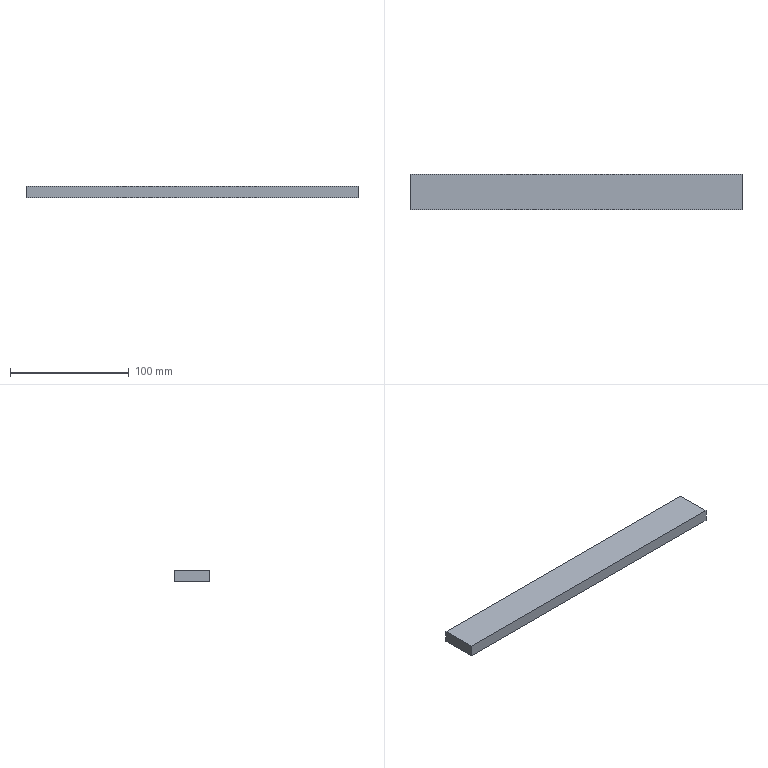Part | NX | features solid 2 | 1 solid | 6 faces | box 279 x 30 x 10 mm | volume 83700 mm3 | plane 6
STEP:
#1=CARTESIAN_POINT('',(-509.173,490.,-20.));
#2=VERTEX_POINT('',#1);
#3=CARTESIAN_POINT('',(-509.173,490.,-30.));
#4=VERTEX_POINT('',#3);
#5=CARTESIAN_POINT('',(-509.173,490.,-10.));
#6=DIRECTION('',(0.,0.,1.));
#7=VECTOR('',#6,1000.);
#8=LINE('',#5,#7);
#9=EDGE_CURVE('',#2,#4,#8,.F.);
#10=ORIENTED_EDGE('',*,*,#9,.F.);
#11=CARTESIAN_POINT('',(-230.173,490.,-20.));
#12=VERTEX_POINT('',#11);
#13=CARTESIAN_POINT('',(-295.173,490.,-20.));
#14=DIRECTION('',(-1.,0.,0.));
#15=VECTOR('',#14,1000.);
#16=LINE('',#13,#15);
#17=EDGE_CURVE('',#12,#2,#16,.T.);
#18=ORIENTED_EDGE('',*,*,#17,.F.);
#19=CARTESIAN_POINT('',(-230.173,490.,-30.));
#20=VERTEX_POINT('',#19);
#21=CARTESIAN_POINT('',(-230.173,490.,-10.));
#22=DIRECTION('',(0.,0.,1.));
#23=VECTOR('',#22,1000.);
#24=LINE('',#21,#23);
#25=EDGE_CURVE('',#12,#20,#24,.F.);
#26=ORIENTED_EDGE('',*,*,#25,.T.);
#27=CARTESIAN_POINT('',(-295.173,490.,-30.));
#28=DIRECTION('',(1.,0.,0.));
#29=VECTOR('',#28,1000.);
#30=LINE('',#27,#29);
#31=EDGE_CURVE('',#20,#4,#30,.F.);
#32=ORIENTED_EDGE('',*,*,#31,.T.);
#33=EDGE_LOOP('',(#10,#18,#26,#32));
#34=FACE_BOUND('',#33,.T.);
#35=CARTESIAN_POINT('',(-295.173,490.,-10.));
#36=DIRECTION('',(0.,-1.,0.));
#37=DIRECTION('',(1.,0.,0.));
#38=AXIS2_PLACEMENT_3D('',#35,#36,#37);
#39=PLANE('',#38);
#40=ADVANCED_FACE('',(#34),#39,.F.);
#41=CARTESIAN_POINT('',(-509.173,460.,-30.));
#42=VERTEX_POINT('',#41);
#43=CARTESIAN_POINT('',(-509.173,460.,-20.));
#44=VERTEX_POINT('',#43);
#45=CARTESIAN_POINT('',(-509.173,460.,-10.));
#46=DIRECTION('',(0.,0.,1.));
#47=VECTOR('',#46,1000.);
#48=LINE('',#45,#47);
#49=EDGE_CURVE('',#42,#44,#48,.T.);
#50=ORIENTED_EDGE('',*,*,#49,.F.);
#51=CARTESIAN_POINT('',(-230.173,460.,-30.));
#52=VERTEX_POINT('',#51);
#53=CARTESIAN_POINT('',(-374.173,460.,-30.));
#54=DIRECTION('',(1.,0.,0.));
#55=VECTOR('',#54,1000.);
#56=LINE('',#53,#55);
#57=EDGE_CURVE('',#42,#52,#56,.T.);
#58=ORIENTED_EDGE('',*,*,#57,.T.);
#59=CARTESIAN_POINT('',(-230.173,460.,-20.));
#60=VERTEX_POINT('',#59);
#61=CARTESIAN_POINT('',(-230.173,460.,-10.));
#62=DIRECTION('',(0.,0.,1.));
#63=VECTOR('',#62,1000.);
#64=LINE('',#61,#63);
#65=EDGE_CURVE('',#52,#60,#64,.T.);
#66=ORIENTED_EDGE('',*,*,#65,.T.);
#67=CARTESIAN_POINT('',(-295.173,460.,-20.));
#68=DIRECTION('',(-1.,0.,0.));
#69=VECTOR('',#68,1000.);
#70=LINE('',#67,#69);
#71=EDGE_CURVE('',#60,#44,#70,.T.);
#72=ORIENTED_EDGE('',*,*,#71,.T.);
#73=EDGE_LOOP('',(#50,#58,#66,#72));
#74=FACE_BOUND('',#73,.T.);
#75=CARTESIAN_POINT('',(-295.173,460.,-10.));
#76=DIRECTION('',(0.,-1.,0.));
#77=DIRECTION('',(1.,0.,0.));
#78=AXIS2_PLACEMENT_3D('',#75,#76,#77);
#79=PLANE('',#78);
#80=ADVANCED_FACE('',(#74),#79,.T.);
#81=ORIENTED_EDGE('',*,*,#65,.F.);
#82=CARTESIAN_POINT('',(-230.173,490.,-30.));
#83=DIRECTION('',(0.,1.,0.));
#84=VECTOR('',#83,1000.);
#85=LINE('',#82,#84);
#86=EDGE_CURVE('',#20,#52,#85,.F.);
#87=ORIENTED_EDGE('',*,*,#86,.F.);
#88=ORIENTED_EDGE('',*,*,#25,.F.);
#89=CARTESIAN_POINT('',(-230.173,460.,-20.));
#90=DIRECTION('',(0.,-1.,0.));
#91=VECTOR('',#90,1000.);
#92=LINE('',#89,#91);
#93=EDGE_CURVE('',#12,#60,#92,.T.);
#94=ORIENTED_EDGE('',*,*,#93,.T.);
#95=EDGE_LOOP('',(#81,#87,#88,#94));
#96=FACE_BOUND('',#95,.T.);
#97=CARTESIAN_POINT('',(-230.173,490.,-10.));
#98=DIRECTION('',(-1.,0.,0.));
#99=DIRECTION('',(0.,0.,1.));
#100=AXIS2_PLACEMENT_3D('',#97,#98,#99);
#101=PLANE('',#100);
#102=ADVANCED_FACE('',(#96),#101,.F.);
#103=CARTESIAN_POINT('',(-509.173,490.,-30.));
#104=DIRECTION('',(0.,1.,0.));
#105=VECTOR('',#104,1000.);
#106=LINE('',#103,#105);
#107=EDGE_CURVE('',#4,#42,#106,.F.);
#108=ORIENTED_EDGE('',*,*,#107,.T.);
#109=ORIENTED_EDGE('',*,*,#49,.T.);
#110=CARTESIAN_POINT('',(-509.173,460.,-20.));
#111=DIRECTION('',(0.,-1.,0.));
#112=VECTOR('',#111,1000.);
#113=LINE('',#110,#112);
#114=EDGE_CURVE('',#2,#44,#113,.T.);
#115=ORIENTED_EDGE('',*,*,#114,.F.);
#116=ORIENTED_EDGE('',*,*,#9,.T.);
#117=EDGE_LOOP('',(#108,#109,#115,#116));
#118=FACE_BOUND('',#117,.T.);
#119=CARTESIAN_POINT('',(-509.173,490.,-10.));
#120=DIRECTION('',(-1.,0.,0.));
#121=DIRECTION('',(0.,0.,1.));
#122=AXIS2_PLACEMENT_3D('',#119,#120,#121);
#123=PLANE('',#122);
#124=ADVANCED_FACE('',(#118),#123,.T.);
#125=ORIENTED_EDGE('',*,*,#57,.F.);
#126=ORIENTED_EDGE('',*,*,#107,.F.);
#127=ORIENTED_EDGE('',*,*,#31,.F.);
#128=ORIENTED_EDGE('',*,*,#86,.T.);
#129=EDGE_LOOP('',(#125,#126,#127,#128));
#130=FACE_BOUND('',#129,.T.);
#131=CARTESIAN_POINT('',(-374.173,460.,-30.));
#132=DIRECTION('',(0.,0.,1.));
#133=DIRECTION('',(1.,0.,0.));
#134=AXIS2_PLACEMENT_3D('',#131,#132,#133);
#135=PLANE('',#134);
#136=ADVANCED_FACE('',(#130),#135,.F.);
#137=ORIENTED_EDGE('',*,*,#114,.T.);
#138=ORIENTED_EDGE('',*,*,#71,.F.);
#139=ORIENTED_EDGE('',*,*,#93,.F.);
#140=ORIENTED_EDGE('',*,*,#17,.T.);
#141=EDGE_LOOP('',(#137,#138,#139,#140));
#142=FACE_BOUND('',#141,.T.);
#143=CARTESIAN_POINT('',(-374.173,460.,-20.));
#144=DIRECTION('',(0.,0.,1.));
#145=DIRECTION('',(1.,0.,0.));
#146=AXIS2_PLACEMENT_3D('',#143,#144,#145);
#147=PLANE('',#146);
#148=ADVANCED_FACE('',(#142),#147,.T.);
#149=CLOSED_SHELL('',(#40,#80,#102,#124,#136,#148));
#150=MANIFOLD_SOLID_BREP('',#149);
#151=(LENGTH_UNIT()NAMED_UNIT(*)SI_UNIT(.MILLI.,.METRE.));
#152=UNCERTAINTY_MEASURE_WITH_UNIT(LENGTH_MEASURE(0.00001),#151,'','');
#153=(NAMED_UNIT(*)PLANE_ANGLE_UNIT()SI_UNIT($,.RADIAN.));
#154=(NAMED_UNIT(*)SI_UNIT($,.STERADIAN.)SOLID_ANGLE_UNIT());
#155=(GEOMETRIC_REPRESENTATION_CONTEXT(3)GLOBAL_UNCERTAINTY_ASSIGNED_CONTEXT((#152))GLOBAL_UNIT_ASSIGNED_CONTEXT((#151,#153,#154))REPRESENTATION_CONTEXT('',''));
#156=ADVANCED_BREP_SHAPE_REPRESENTATION('',(#150),#155);